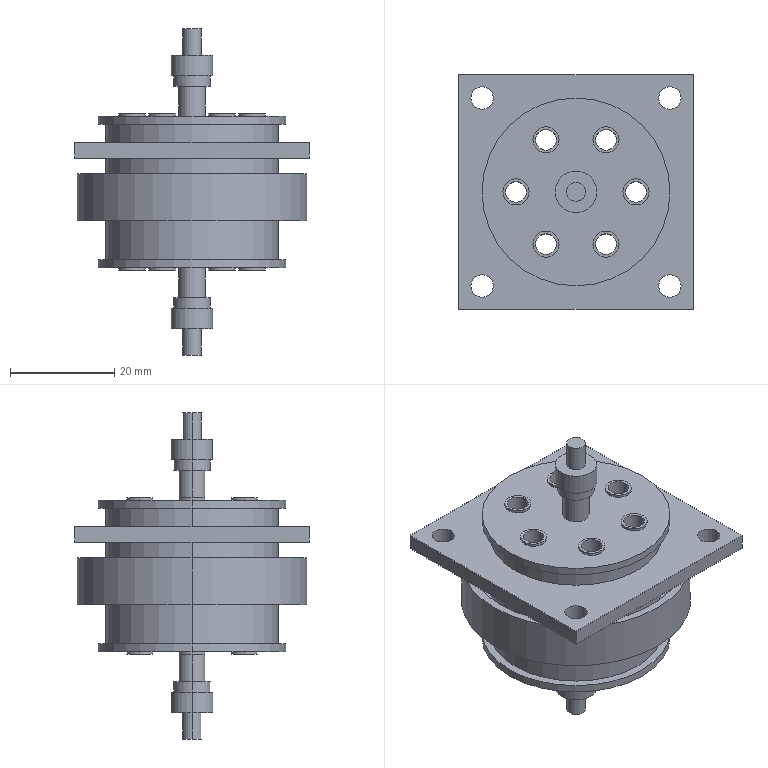Part | NX | features BREP 1 | 1 solid | 144 faces | box 45 x 45 x 62.5 mm | volume 25262 mm3 | cylinder 102 | plane 42 | commonest cylinder face diameters 5 x40 4 x24 4.3 x8 33 x6 36 x6 3.6 x4